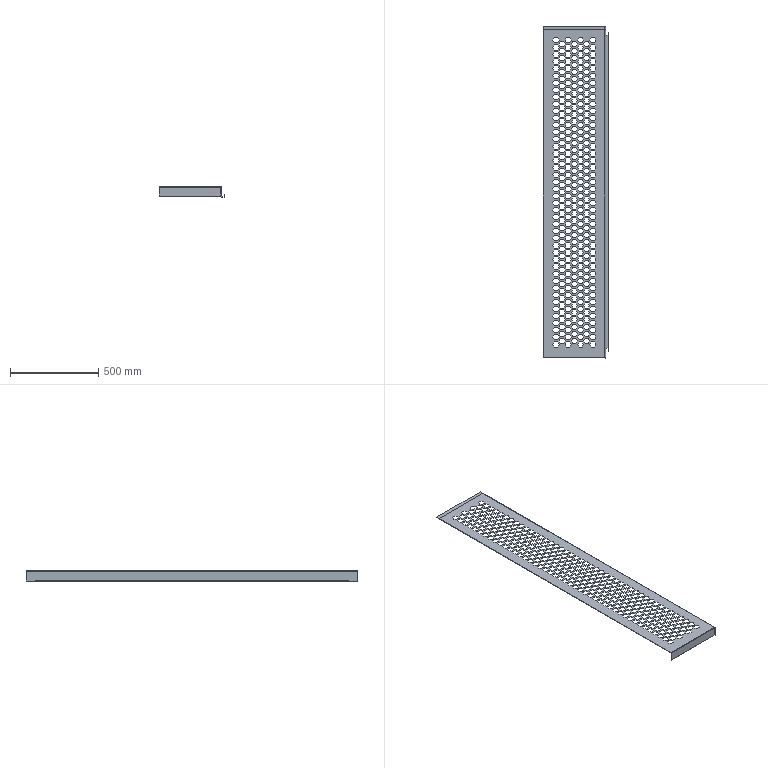Part | SolidWorks | features BaseBody 1 | 1 solid | 1885 faces | box 370 x 1878 x 57 mm | volume 1188776 mm3 | plane 1870 | cylinder 11 | torus 4 | commonest cylinder face diameters 6 x5 2 x4 30 x2